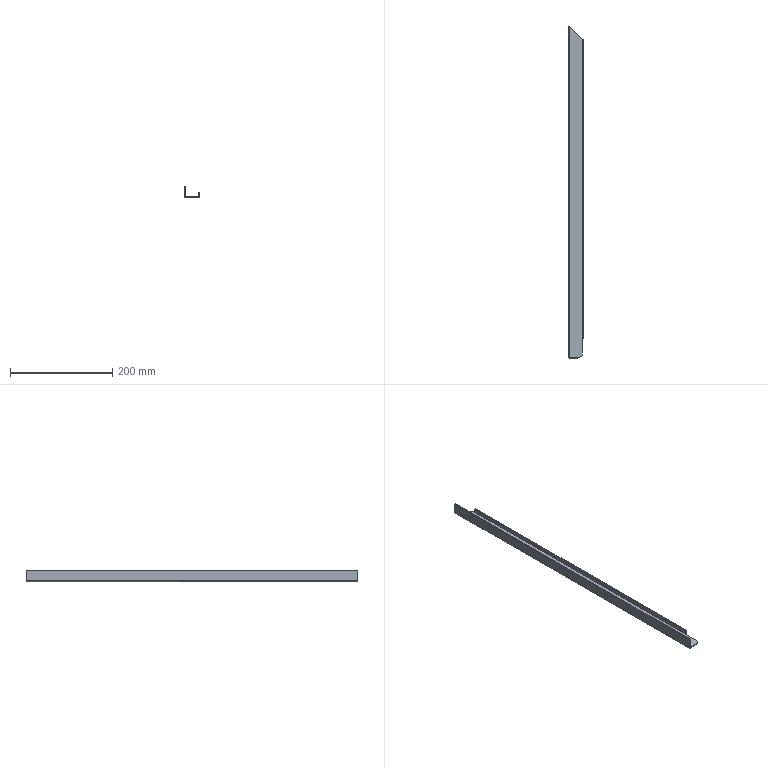Part | STEP file | Rear Closing Plate Door Frame Right | 1 solid | 21 faces | box 30 x 650.24 x 22 mm | volume 72183 mm3 | plane 14 | cylinder 5 | spline 2 | commonest cylinder face diameters 0.2 x2 4.2 x2 20 x1
STEP:
#1=CARTESIAN_POINT('',(24.549,-282.608,2.));
#2=VERTEX_POINT('',#1);
#3=CARTESIAN_POINT('',(14.549,-292.608,2.));
#4=VERTEX_POINT('',#3);
#5=CARTESIAN_POINT('',(14.549,-282.608,2.));
#6=DIRECTION('',(0.,0.,-1.));
#7=DIRECTION('',(-1.,0.,0.));
#8=AXIS2_PLACEMENT_3D('',#5,#6,#7);
#9=CIRCLE('',#8,10.);
#10=EDGE_CURVE('',#2,#4,#9,.T.);
#11=ORIENTED_EDGE('',*,*,#10,.F.);
#12=CARTESIAN_POINT('',(24.549,-254.608,2.));
#13=VERTEX_POINT('',#12);
#14=CARTESIAN_POINT('',(24.549,0.,2.));
#15=DIRECTION('',(0.,-1.,0.));
#16=VECTOR('',#15,1000.);
#17=LINE('',#14,#16);
#18=EDGE_CURVE('',#13,#2,#17,.T.);
#19=ORIENTED_EDGE('',*,*,#18,.F.);
#20=CARTESIAN_POINT('',(24.649,-254.608,2.));
#21=VERTEX_POINT('',#20);
#22=CARTESIAN_POINT('',(667.249,-254.608,2.));
#23=DIRECTION('',(1.,0.,0.));
#24=VECTOR('',#23,1000.);
#25=LINE('',#22,#24);
#26=EDGE_CURVE('',#13,#21,#25,.T.);
#27=ORIENTED_EDGE('',*,*,#26,.T.);
#28=CARTESIAN_POINT('',(24.649,331.492,2.));
#29=VERTEX_POINT('',#28);
#30=CARTESIAN_POINT('',(24.649,0.,2.));
#31=DIRECTION('',(0.,-1.,0.));
#32=VECTOR('',#31,1000.);
#33=LINE('',#30,#32);
#34=EDGE_CURVE('',#29,#21,#33,.T.);
#35=ORIENTED_EDGE('',*,*,#34,.F.);
#36=CARTESIAN_POINT('',(-1.151,357.292,2.));
#37=VERTEX_POINT('',#36);
#38=CARTESIAN_POINT('',(-1.151,357.292,2.));
#39=DIRECTION('',(0.7071,-0.7071,0.));
#40=VECTOR('',#39,1000.);
#41=LINE('',#38,#40);
#42=EDGE_CURVE('',#37,#29,#41,.T.);
#43=ORIENTED_EDGE('',*,*,#42,.F.);
#44=CARTESIAN_POINT('',(-1.151,-292.608,2.));
#45=VERTEX_POINT('',#44);
#46=CARTESIAN_POINT('',(-1.151,0.,2.));
#47=DIRECTION('',(0.,1.,0.));
#48=VECTOR('',#47,1000.);
#49=LINE('',#46,#48);
#50=EDGE_CURVE('',#45,#37,#49,.T.);
#51=ORIENTED_EDGE('',*,*,#50,.F.);
#52=CARTESIAN_POINT('',(0.,-292.608,2.));
#53=DIRECTION('',(-1.,0.,0.));
#54=VECTOR('',#53,1000.);
#55=LINE('',#52,#54);
#56=EDGE_CURVE('',#4,#45,#55,.T.);
#57=ORIENTED_EDGE('',*,*,#56,.F.);
#58=EDGE_LOOP('',(#11,#19,#27,#35,#43,#51,#57));
#59=FACE_OUTER_BOUND('',#58,.T.);
#60=CARTESIAN_POINT('',(0.,0.,2.));
#61=DIRECTION('',(0.,0.,-1.));
#62=DIRECTION('',(-1.,0.,0.));
#63=AXIS2_PLACEMENT_3D('',#60,#61,#62);
#64=PLANE('',#63);
#65=ADVANCED_FACE('',(#59),#64,.F.);
#66=CARTESIAN_POINT('',(14.549,-292.608,0.));
#67=VERTEX_POINT('',#66);
#68=CARTESIAN_POINT('',(14.549,-292.608,0.));
#69=DIRECTION('',(0.,0.,-1.));
#70=VECTOR('',#69,1000.);
#71=LINE('',#68,#70);
#72=EDGE_CURVE('',#4,#67,#71,.T.);
#73=ORIENTED_EDGE('',*,*,#72,.F.);
#74=ORIENTED_EDGE('',*,*,#56,.T.);
#75=CARTESIAN_POINT('',(-1.251,-292.608,2.1));
#76=VERTEX_POINT('',#75);
#77=CARTESIAN_POINT('',(-1.151,-292.608,2.1));
#78=DIRECTION('',(0.,1.,0.));
#79=DIRECTION('',(-1.,0.,0.));
#80=AXIS2_PLACEMENT_3D('',#77,#78,#79);
#81=CIRCLE('',#80,0.1);
#82=EDGE_CURVE('',#45,#76,#81,.T.);
#83=ORIENTED_EDGE('',*,*,#82,.T.);
#84=CARTESIAN_POINT('',(-1.251,-292.608,22.));
#85=VERTEX_POINT('',#84);
#86=CARTESIAN_POINT('',(-1.251,-292.608,22.));
#87=DIRECTION('',(0.,0.,-1.));
#88=VECTOR('',#87,1000.);
#89=LINE('',#86,#88);
#90=EDGE_CURVE('',#85,#76,#89,.T.);
#91=ORIENTED_EDGE('',*,*,#90,.F.);
#92=CARTESIAN_POINT('',(-3.251,-292.608,22.));
#93=VERTEX_POINT('',#92);
#94=CARTESIAN_POINT('',(-3.251,-292.608,22.));
#95=DIRECTION('',(-1.,0.,0.));
#96=VECTOR('',#95,1000.);
#97=LINE('',#94,#96);
#98=EDGE_CURVE('',#85,#93,#97,.T.);
#99=ORIENTED_EDGE('',*,*,#98,.T.);
#100=CARTESIAN_POINT('',(-3.251,-292.608,2.1));
#101=VERTEX_POINT('',#100);
#102=CARTESIAN_POINT('',(-3.251,-292.608,22.));
#103=DIRECTION('',(0.,0.,-1.));
#104=VECTOR('',#103,1000.);
#105=LINE('',#102,#104);
#106=EDGE_CURVE('',#93,#101,#105,.T.);
#107=ORIENTED_EDGE('',*,*,#106,.T.);
#108=CARTESIAN_POINT('',(-1.151,-292.608,0.));
#109=VERTEX_POINT('',#108);
#110=CARTESIAN_POINT('',(-1.151,-292.608,2.1));
#111=DIRECTION('',(0.,1.,0.));
#112=DIRECTION('',(-1.,0.,0.));
#113=AXIS2_PLACEMENT_3D('',#110,#111,#112);
#114=CIRCLE('',#113,2.1);
#115=EDGE_CURVE('',#109,#101,#114,.T.);
#116=ORIENTED_EDGE('',*,*,#115,.F.);
#117=CARTESIAN_POINT('',(24.549,-292.608,0.));
#118=DIRECTION('',(-1.,0.,0.));
#119=VECTOR('',#118,1000.);
#120=LINE('',#117,#119);
#121=EDGE_CURVE('',#67,#109,#120,.T.);
#122=ORIENTED_EDGE('',*,*,#121,.F.);
#123=EDGE_LOOP('',(#73,#74,#83,#91,#99,#107,#116,#122));
#124=FACE_OUTER_BOUND('',#123,.T.);
#125=CARTESIAN_POINT('',(24.549,-292.608,0.));
#126=DIRECTION('',(0.,1.,0.));
#127=DIRECTION('',(-1.,0.,0.));
#128=AXIS2_PLACEMENT_3D('',#125,#126,#127);
#129=PLANE('',#128);
#130=ADVANCED_FACE('',(#124),#129,.F.);
#131=CARTESIAN_POINT('',(24.549,-282.608,0.));
#132=VERTEX_POINT('',#131);
#133=CARTESIAN_POINT('',(14.549,-282.608,0.));
#134=DIRECTION('',(0.,0.,1.));
#135=DIRECTION('',(-1.,0.,0.));
#136=AXIS2_PLACEMENT_3D('',#133,#134,#135);
#137=CIRCLE('',#136,10.);
#138=EDGE_CURVE('',#67,#132,#137,.T.);
#139=ORIENTED_EDGE('',*,*,#138,.T.);
#140=CARTESIAN_POINT('',(24.549,-282.608,0.));
#141=DIRECTION('',(0.,0.,1.));
#142=VECTOR('',#141,1000.);
#143=LINE('',#140,#142);
#144=EDGE_CURVE('',#132,#2,#143,.T.);
#145=ORIENTED_EDGE('',*,*,#144,.T.);
#146=ORIENTED_EDGE('',*,*,#10,.T.);
#147=ORIENTED_EDGE('',*,*,#72,.T.);
#148=EDGE_LOOP('',(#139,#145,#146,#147));
#149=FACE_OUTER_BOUND('',#148,.T.);
#150=CARTESIAN_POINT('',(14.549,-282.608,0.));
#151=DIRECTION('',(0.,0.,-1.));
#152=DIRECTION('',(-1.,0.,0.));
#153=AXIS2_PLACEMENT_3D('',#150,#151,#152);
#154=CYLINDRICAL_SURFACE('',#153,10.);
#155=ADVANCED_FACE('',(#149),#154,.T.);
#156=ORIENTED_EDGE('',*,*,#144,.F.);
#157=CARTESIAN_POINT('',(24.549,-254.608,0.));
#158=VERTEX_POINT('',#157);
#159=CARTESIAN_POINT('',(24.549,-254.608,0.));
#160=DIRECTION('',(0.,-1.,0.));
#161=VECTOR('',#160,1000.);
#162=LINE('',#159,#161);
#163=EDGE_CURVE('',#158,#132,#162,.T.);
#164=ORIENTED_EDGE('',*,*,#163,.F.);
#165=CARTESIAN_POINT('',(24.549,-254.608,0.));
#166=DIRECTION('',(0.,0.,-1.));
#167=VECTOR('',#166,1000.);
#168=LINE('',#165,#167);
#169=EDGE_CURVE('',#13,#158,#168,.T.);
#170=ORIENTED_EDGE('',*,*,#169,.F.);
#171=ORIENTED_EDGE('',*,*,#18,.T.);
#172=EDGE_LOOP('',(#156,#164,#170,#171));
#173=FACE_OUTER_BOUND('',#172,.T.);
#174=CARTESIAN_POINT('',(24.549,-254.608,0.));
#175=DIRECTION('',(-1.,0.,0.));
#176=DIRECTION('',(0.,-1.,0.));
#177=AXIS2_PLACEMENT_3D('',#174,#175,#176);
#178=PLANE('',#177);
#179=ADVANCED_FACE('',(#173),#178,.F.);
#180=ORIENTED_EDGE('',*,*,#34,.T.);
#181=CARTESIAN_POINT('',(24.749,-254.608,2.1));
#182=VERTEX_POINT('',#181);
#183=CARTESIAN_POINT('',(24.649,-254.608,2.1));
#184=DIRECTION('',(0.,1.,0.));
#185=DIRECTION('',(1.,0.,0.));
#186=AXIS2_PLACEMENT_3D('',#183,#184,#185);
#187=CIRCLE('',#186,0.1);
#188=EDGE_CURVE('',#182,#21,#187,.T.);
#189=ORIENTED_EDGE('',*,*,#188,.F.);
#190=CARTESIAN_POINT('',(24.749,329.392,2.1));
#191=VERTEX_POINT('',#190);
#192=CARTESIAN_POINT('',(24.749,0.,2.1));
#193=DIRECTION('',(0.,-1.,0.));
#194=VECTOR('',#193,1000.);
#195=LINE('',#192,#194);
#196=EDGE_CURVE('',#191,#182,#195,.T.);
#197=ORIENTED_EDGE('',*,*,#196,.F.);
#198=CARTESIAN_POINT('',(24.649,331.492,2.));
#199=CARTESIAN_POINT('',(24.716,330.092,2.));
#200=CARTESIAN_POINT('',(24.749,329.392,2.05));
#201=CARTESIAN_POINT('',(24.749,329.392,2.1));
#202=(BOUNDED_CURVE()B_SPLINE_CURVE(3,(#198,#199,#200,#201),.UNSPECIFIED.,.F.,.F.)B_SPLINE_CURVE_WITH_KNOTS((4,4),(0.,0.002112),.UNSPECIFIED.)CURVE()GEOMETRIC_REPRESENTATION_ITEM()RATIONAL_B_SPLINE_CURVE((0.5,0.5,0.6667,1.))REPRESENTATION_ITEM(''));
#203=EDGE_CURVE('',#29,#191,#202,.T.);
#204=ORIENTED_EDGE('',*,*,#203,.F.);
#205=EDGE_LOOP('',(#180,#189,#197,#204));
#206=FACE_OUTER_BOUND('',#205,.T.);
#207=CARTESIAN_POINT('',(24.649,0.,2.1));
#208=DIRECTION('',(0.,-1.,0.));
#209=DIRECTION('',(1.,0.,0.));
#210=AXIS2_PLACEMENT_3D('',#207,#208,#209);
#211=CYLINDRICAL_SURFACE('',#210,0.1);
#212=ADVANCED_FACE('',(#206),#211,.F.);
#213=ORIENTED_EDGE('',*,*,#42,.T.);
#214=CARTESIAN_POINT('',(24.649,331.492,0.));
#215=VERTEX_POINT('',#214);
#216=CARTESIAN_POINT('',(24.649,331.492,0.));
#217=DIRECTION('',(0.,0.,1.));
#218=VECTOR('',#217,1000.);
#219=LINE('',#216,#218);
#220=EDGE_CURVE('',#215,#29,#219,.T.);
#221=ORIENTED_EDGE('',*,*,#220,.F.);
#222=CARTESIAN_POINT('',(-1.151,357.292,0.));
#223=VERTEX_POINT('',#222);
#224=CARTESIAN_POINT('',(-1.251,357.392,0.));
#225=DIRECTION('',(0.7071,-0.7071,0.));
#226=VECTOR('',#225,1000.);
#227=LINE('',#224,#226);
#228=EDGE_CURVE('',#223,#215,#227,.T.);
#229=ORIENTED_EDGE('',*,*,#228,.F.);
#230=CARTESIAN_POINT('',(-1.151,357.292,0.));
#231=DIRECTION('',(0.,0.,-1.));
#232=VECTOR('',#231,1000.);
#233=LINE('',#230,#232);
#234=EDGE_CURVE('',#37,#223,#233,.T.);
#235=ORIENTED_EDGE('',*,*,#234,.F.);
#236=EDGE_LOOP('',(#213,#221,#229,#235));
#237=FACE_OUTER_BOUND('',#236,.T.);
#238=CARTESIAN_POINT('',(-1.251,357.392,0.));
#239=DIRECTION('',(-0.7071,-0.7071,0.));
#240=DIRECTION('',(0.7071,-0.7071,0.));
#241=AXIS2_PLACEMENT_3D('',#238,#239,#240);
#242=PLANE('',#241);
#243=ADVANCED_FACE('',(#237),#242,.F.);
#244=CARTESIAN_POINT('',(-1.251,357.392,2.1));
#245=VERTEX_POINT('',#244);
#246=CARTESIAN_POINT('',(-1.251,359.392,2.1));
#247=DIRECTION('',(0.,1.,0.));
#248=VECTOR('',#247,1000.);
#249=LINE('',#246,#248);
#250=EDGE_CURVE('',#76,#245,#249,.T.);
#251=ORIENTED_EDGE('',*,*,#250,.F.);
#252=ORIENTED_EDGE('',*,*,#82,.F.);
#253=ORIENTED_EDGE('',*,*,#50,.T.);
#254=CARTESIAN_POINT('',(-1.251,357.392,2.1));
#255=CARTESIAN_POINT('',(-1.251,357.392,2.093));
#256=CARTESIAN_POINT('',(-1.251,357.399,2.09));
#257=CARTESIAN_POINT('',(-1.25,357.41,2.084));
#258=CARTESIAN_POINT('',(-1.249,357.416,2.081));
#259=CARTESIAN_POINT('',(-1.248,357.434,2.074));
#260=CARTESIAN_POINT('',(-1.247,357.446,2.07));
#261=CARTESIAN_POINT('',(-1.243,357.483,2.059));
#262=CARTESIAN_POINT('',(-1.239,357.508,2.052));
#263=CARTESIAN_POINT('',(-1.231,357.557,2.039));
#264=CARTESIAN_POINT('',(-1.226,357.581,2.033));
#265=CARTESIAN_POINT('',(-1.216,357.611,2.024));
#266=CARTESIAN_POINT('',(-1.214,357.616,2.022));
#267=CARTESIAN_POINT('',(-1.208,357.627,2.017));
#268=CARTESIAN_POINT('',(-1.203,357.633,2.014));
#269=CARTESIAN_POINT('',(-1.192,357.628,2.009));
#270=CARTESIAN_POINT('',(-1.189,357.622,2.008));
#271=CARTESIAN_POINT('',(-1.185,357.61,2.006));
#272=CARTESIAN_POINT('',(-1.183,357.604,2.005));
#273=CARTESIAN_POINT('',(-1.168,357.548,2.001));
#274=CARTESIAN_POINT('',(-1.165,357.496,2.001));
#275=CARTESIAN_POINT('',(-1.157,357.394,2.));
#276=CARTESIAN_POINT('',(-1.154,357.343,2.));
#277=CARTESIAN_POINT('',(-1.151,357.292,2.));
#278=B_SPLINE_CURVE_WITH_KNOTS('',3,(#254,#255,#256,#257,#258,#259,#260,#261,#262,#263,#264,#265,#266,#267,#268,#269,#270,#271,#272,#273,#274,#275,#276,#277),.UNSPECIFIED.,.F.,.F.,(4,2,2,2,2,2,2,2,2,2,2,4),(0.,0.00001954,0.00003907,0.00007815,0.0001563,0.0002344,0.000254,0.0002735,0.0002931,0.0003126,0.0004689,0.0006252),.UNSPECIFIED.);
#279=EDGE_CURVE('',#245,#37,#278,.T.);
#280=ORIENTED_EDGE('',*,*,#279,.F.);
#281=EDGE_LOOP('',(#251,#252,#253,#280));
#282=FACE_OUTER_BOUND('',#281,.T.);
#283=CARTESIAN_POINT('',(-1.151,359.392,2.1));
#284=DIRECTION('',(0.,1.,0.));
#285=DIRECTION('',(-1.,0.,0.));
#286=AXIS2_PLACEMENT_3D('',#283,#284,#285);
#287=CYLINDRICAL_SURFACE('',#286,0.1);
#288=ADVANCED_FACE('',(#282),#287,.F.);
#289=CARTESIAN_POINT('',(24.649,-254.608,0.));
#290=VERTEX_POINT('',#289);
#291=CARTESIAN_POINT('',(24.649,0.,0.));
#292=DIRECTION('',(0.,-1.,0.));
#293=VECTOR('',#292,1000.);
#294=LINE('',#291,#293);
#295=EDGE_CURVE('',#215,#290,#294,.T.);
#296=ORIENTED_EDGE('',*,*,#295,.T.);
#297=CARTESIAN_POINT('',(0.,-254.608,0.));
#298=DIRECTION('',(-1.,0.,0.));
#299=VECTOR('',#298,1000.);
#300=LINE('',#297,#299);
#301=EDGE_CURVE('',#290,#158,#300,.T.);
#302=ORIENTED_EDGE('',*,*,#301,.T.);
#303=ORIENTED_EDGE('',*,*,#163,.T.);
#304=ORIENTED_EDGE('',*,*,#138,.F.);
#305=ORIENTED_EDGE('',*,*,#121,.T.);
#306=CARTESIAN_POINT('',(-1.151,0.,0.));
#307=DIRECTION('',(0.,1.,0.));
#308=VECTOR('',#307,1000.);
#309=LINE('',#306,#308);
#310=EDGE_CURVE('',#109,#223,#309,.T.);
#311=ORIENTED_EDGE('',*,*,#310,.T.);
#312=ORIENTED_EDGE('',*,*,#228,.T.);
#313=EDGE_LOOP('',(#296,#302,#303,#304,#305,#311,#312));
#314=FACE_OUTER_BOUND('',#313,.T.);
#315=CARTESIAN_POINT('',(0.,0.,0.));
#316=DIRECTION('',(0.,0.,-1.));
#317=DIRECTION('',(-1.,0.,0.));
#318=AXIS2_PLACEMENT_3D('',#315,#316,#317);
#319=PLANE('',#318);
#320=ADVANCED_FACE('',(#314),#319,.T.);
#321=ORIENTED_EDGE('',*,*,#26,.F.);
#322=ORIENTED_EDGE('',*,*,#169,.T.);
#323=ORIENTED_EDGE('',*,*,#301,.F.);
#324=CARTESIAN_POINT('',(26.749,-254.608,2.1));
#325=VERTEX_POINT('',#324);
#326=CARTESIAN_POINT('',(24.649,-254.608,2.1));
#327=DIRECTION('',(0.,1.,0.));
#328=DIRECTION('',(1.,0.,0.));
#329=AXIS2_PLACEMENT_3D('',#326,#327,#328);
#330=CIRCLE('',#329,2.1);
#331=EDGE_CURVE('',#325,#290,#330,.T.);
#332=ORIENTED_EDGE('',*,*,#331,.F.);
#333=CARTESIAN_POINT('',(26.749,-254.608,10.));
#334=VERTEX_POINT('',#333);
#335=CARTESIAN_POINT('',(26.749,-254.608,22.));
#336=DIRECTION('',(0.,0.,1.));
#337=VECTOR('',#336,1000.);
#338=LINE('',#335,#337);
#339=EDGE_CURVE('',#325,#334,#338,.T.);
#340=ORIENTED_EDGE('',*,*,#339,.T.);
#341=CARTESIAN_POINT('',(24.749,-254.608,10.));
#342=VERTEX_POINT('',#341);
#343=CARTESIAN_POINT('',(26.749,-254.608,10.));
#344=DIRECTION('',(-1.,0.,0.));
#345=VECTOR('',#344,1000.);
#346=LINE('',#343,#345);
#347=EDGE_CURVE('',#334,#342,#346,.T.);
#348=ORIENTED_EDGE('',*,*,#347,.T.);
#349=CARTESIAN_POINT('',(24.749,-254.608,22.));
#350=DIRECTION('',(0.,0.,-1.));
#351=VECTOR('',#350,1000.);
#352=LINE('',#349,#351);
#353=EDGE_CURVE('',#342,#182,#352,.T.);
#354=ORIENTED_EDGE('',*,*,#353,.T.);
#355=ORIENTED_EDGE('',*,*,#188,.T.);
#356=EDGE_LOOP('',(#321,#322,#323,#332,#340,#348,#354,#355));
#357=FACE_OUTER_BOUND('',#356,.T.);
#358=CARTESIAN_POINT('',(667.249,-254.608,0.));
#359=DIRECTION('',(0.,1.,0.));
#360=DIRECTION('',(0.,0.,1.));
#361=AXIS2_PLACEMENT_3D('',#358,#359,#360);
#362=PLANE('',#361);
#363=ADVANCED_FACE('',(#357),#362,.F.);
#364=ORIENTED_EDGE('',*,*,#203,.T.);
#365=CARTESIAN_POINT('',(26.749,329.392,2.1));
#366=VERTEX_POINT('',#365);
#367=CARTESIAN_POINT('',(25.749,329.392,2.1));
#368=DIRECTION('',(-1.,0.,0.));
#369=VECTOR('',#368,1000.);
#370=LINE('',#367,#369);
#371=EDGE_CURVE('',#366,#191,#370,.T.);
#372=ORIENTED_EDGE('',*,*,#371,.F.);
#373=CARTESIAN_POINT('',(24.649,331.492,0.));
#374=CARTESIAN_POINT('',(26.049,330.092,0.));
#375=CARTESIAN_POINT('',(26.749,329.392,1.05));
#376=CARTESIAN_POINT('',(26.749,329.392,2.1));
#377=(BOUNDED_CURVE()B_SPLINE_CURVE(3,(#373,#374,#375,#376),.UNSPECIFIED.,.F.,.F.)B_SPLINE_CURVE_WITH_KNOTS((4,4),(0.,0.003971),.UNSPECIFIED.)CURVE()GEOMETRIC_REPRESENTATION_ITEM()RATIONAL_B_SPLINE_CURVE((0.5,0.5,0.6667,1.))REPRESENTATION_ITEM(''));
#378=EDGE_CURVE('',#215,#366,#377,.T.);
#379=ORIENTED_EDGE('',*,*,#378,.F.);
#380=ORIENTED_EDGE('',*,*,#220,.T.);
#381=EDGE_LOOP('',(#364,#372,#379,#380));
#382=FACE_OUTER_BOUND('',#381,.T.);
#383=CARTESIAN_POINT('',(26.749,329.392,2.1));
#384=CARTESIAN_POINT('',(26.082,329.392,2.1));
#385=CARTESIAN_POINT('',(25.416,329.392,2.1));
#386=CARTESIAN_POINT('',(24.749,329.392,2.1));
#387=CARTESIAN_POINT('',(26.749,329.392,6.3));
#388=CARTESIAN_POINT('',(26.082,329.392,4.967));
#389=CARTESIAN_POINT('',(25.416,329.392,3.633));
#390=CARTESIAN_POINT('',(24.749,329.392,2.3));
#391=CARTESIAN_POINT('',(22.549,333.592,6.3));
#392=CARTESIAN_POINT('',(23.216,333.592,4.967));
#393=CARTESIAN_POINT('',(23.882,333.592,3.633));
#394=CARTESIAN_POINT('',(24.549,333.592,2.3));
#395=CARTESIAN_POINT('',(22.549,333.592,2.1));
#396=CARTESIAN_POINT('',(23.216,333.592,2.1));
#397=CARTESIAN_POINT('',(23.882,333.592,2.1));
#398=CARTESIAN_POINT('',(24.549,333.592,2.1));
#399=CARTESIAN_POINT('',(22.549,333.592,-2.1));
#400=CARTESIAN_POINT('',(23.216,333.592,-0.7667));
#401=CARTESIAN_POINT('',(23.882,333.592,0.5667));
#402=CARTESIAN_POINT('',(24.549,333.592,1.9));
#403=CARTESIAN_POINT('',(26.749,329.392,-2.1));
#404=CARTESIAN_POINT('',(26.082,329.392,-0.7667));
#405=CARTESIAN_POINT('',(25.416,329.392,0.5667));
#406=CARTESIAN_POINT('',(24.749,329.392,1.9));
#407=CARTESIAN_POINT('',(26.749,329.392,2.1));
#408=CARTESIAN_POINT('',(26.082,329.392,2.1));
#409=CARTESIAN_POINT('',(25.416,329.392,2.1));
#410=CARTESIAN_POINT('',(24.749,329.392,2.1));
#411=(BOUNDED_SURFACE()B_SPLINE_SURFACE(3,3,((#383,#384,#385,#386),(#387,#388,#389,#390),(#391,#392,#393,#394),(#395,#396,#397,#398),(#399,#400,#401,#402),(#403,#404,#405,#406),(#407,#408,#409,#410)),.UNSPECIFIED.,.T.,.F.,.F.)B_SPLINE_SURFACE_WITH_KNOTS((4,3,4),(4,4),(0.,0.5,1.),(0.,1.),.UNSPECIFIED.)GEOMETRIC_REPRESENTATION_ITEM()RATIONAL_B_SPLINE_SURFACE(((1.,1.,1.,1.),(0.3333,0.3333,0.3333,0.3333),(0.3333,0.3333,0.3333,0.3333),(1.,1.,1.,1.),(0.3333,0.3333,0.3333,0.3333),(0.3333,0.3333,0.3333,0.3333),(1.,1.,1.,1.)))REPRESENTATION_ITEM('')SURFACE());
#412=ADVANCED_FACE('',(#382),#411,.F.);
#413=CARTESIAN_POINT('',(24.749,329.392,10.));
#414=VERTEX_POINT('',#413);
#415=CARTESIAN_POINT('',(24.749,329.392,10.));
#416=DIRECTION('',(0.,-1.,0.));
#417=VECTOR('',#416,1000.);
#418=LINE('',#415,#417);
#419=EDGE_CURVE('',#414,#342,#418,.T.);
#420=ORIENTED_EDGE('',*,*,#419,.F.);
#421=CARTESIAN_POINT('',(24.749,329.392,22.));
#422=DIRECTION('',(0.,0.,1.));
#423=VECTOR('',#422,1000.);
#424=LINE('',#421,#423);
#425=EDGE_CURVE('',#191,#414,#424,.T.);
#426=ORIENTED_EDGE('',*,*,#425,.F.);
#427=ORIENTED_EDGE('',*,*,#196,.T.);
#428=ORIENTED_EDGE('',*,*,#353,.F.);
#429=EDGE_LOOP('',(#420,#426,#427,#428));
#430=FACE_OUTER_BOUND('',#429,.T.);
#431=CARTESIAN_POINT('',(24.749,329.392,22.));
#432=DIRECTION('',(1.,0.,0.));
#433=DIRECTION('',(0.,1.,0.));
#434=AXIS2_PLACEMENT_3D('',#431,#432,#433);
#435=PLANE('',#434);
#436=ADVANCED_FACE('',(#430),#435,.F.);
#437=ORIENTED_EDGE('',*,*,#279,.T.);
#438=ORIENTED_EDGE('',*,*,#234,.T.);
#439=CARTESIAN_POINT('',(-3.251,357.392,2.1));
#440=VERTEX_POINT('',#439);
#441=CARTESIAN_POINT('',(-3.251,357.392,2.1));
#442=CARTESIAN_POINT('',(-3.251,357.392,1.958));
#443=CARTESIAN_POINT('',(-3.237,357.403,1.816));
#444=CARTESIAN_POINT('',(-3.18,357.435,1.539));
#445=CARTESIAN_POINT('',(-3.138,357.455,1.406));
#446=CARTESIAN_POINT('',(-3.029,357.497,1.15));
#447=CARTESIAN_POINT('',(-2.961,357.519,1.026));
#448=CARTESIAN_POINT('',(-2.803,357.561,0.796));
#449=CARTESIAN_POINT('',(-2.713,357.58,0.6898));
#450=CARTESIAN_POINT('',(-2.513,357.612,0.495));
#451=CARTESIAN_POINT('',(-2.4,357.624,0.4061));
#452=CARTESIAN_POINT('',(-2.163,357.634,0.2546));
#453=CARTESIAN_POINT('',(-2.036,357.632,0.1903));
#454=CARTESIAN_POINT('',(-1.773,357.6,0.08907));
#455=CARTESIAN_POINT('',(-1.637,357.572,0.05272));
#456=CARTESIAN_POINT('',(-1.376,357.468,0.00789));
#457=CARTESIAN_POINT('',(-1.253,357.393,0.));
#458=CARTESIAN_POINT('',(-1.151,357.292,0.));
#459=B_SPLINE_CURVE_WITH_KNOTS('',3,(#441,#442,#443,#444,#445,#446,#447,#448,#449,#450,#451,#452,#453,#454,#455,#456,#457,#458),.UNSPECIFIED.,.F.,.F.,(4,2,2,2,2,2,2,2,4),(0.,0.0004273,0.0008547,0.001282,0.001709,0.002137,0.002564,0.002991,0.003419),.UNSPECIFIED.);
#460=EDGE_CURVE('',#440,#223,#459,.T.);
#461=ORIENTED_EDGE('',*,*,#460,.F.);
#462=CARTESIAN_POINT('',(-2.251,357.392,2.1));
#463=DIRECTION('',(-1.,0.,0.));
#464=VECTOR('',#463,1000.);
#465=LINE('',#462,#464);
#466=EDGE_CURVE('',#245,#440,#465,.T.);
#467=ORIENTED_EDGE('',*,*,#466,.F.);
#468=EDGE_LOOP('',(#437,#438,#461,#467));
#469=FACE_OUTER_BOUND('',#468,.T.);
#470=CARTESIAN_POINT('',(-1.151,357.292,-0.0202));
#471=CARTESIAN_POINT('',(-1.328,357.466,-0.0202));
#472=CARTESIAN_POINT('',(-1.564,357.561,0.003288));
#473=CARTESIAN_POINT('',(-2.071,357.645,0.1713));
#474=CARTESIAN_POINT('',(-2.341,357.636,0.3179));
#475=CARTESIAN_POINT('',(-2.801,357.573,0.7325));
#476=CARTESIAN_POINT('',(-2.988,357.52,0.999));
#477=CARTESIAN_POINT('',(-3.224,357.429,1.559));
#478=CARTESIAN_POINT('',(-3.271,357.392,1.851));
#479=CARTESIAN_POINT('',(-3.271,357.392,2.1));
#480=CARTESIAN_POINT('',(-1.151,357.292,0.));
#481=CARTESIAN_POINT('',(-1.326,357.466,0.));
#482=CARTESIAN_POINT('',(-1.56,357.561,0.02326));
#483=CARTESIAN_POINT('',(-2.063,357.645,0.1897));
#484=CARTESIAN_POINT('',(-2.329,357.636,0.3349));
#485=CARTESIAN_POINT('',(-2.785,357.573,0.7455));
#486=CARTESIAN_POINT('',(-2.971,357.52,1.01));
#487=CARTESIAN_POINT('',(-3.204,357.429,1.565));
#488=CARTESIAN_POINT('',(-3.251,357.392,1.853));
#489=CARTESIAN_POINT('',(-3.251,357.392,2.1));
#490=CARTESIAN_POINT('',(-1.151,357.292,2.));
#491=CARTESIAN_POINT('',(-1.16,357.467,2.));
#492=CARTESIAN_POINT('',(-1.171,357.561,2.001));
#493=CARTESIAN_POINT('',(-1.195,357.645,2.009));
#494=CARTESIAN_POINT('',(-1.207,357.636,2.016));
#495=CARTESIAN_POINT('',(-1.229,357.573,2.035));
#496=CARTESIAN_POINT('',(-1.238,357.52,2.048));
#497=CARTESIAN_POINT('',(-1.249,357.429,2.075));
#498=CARTESIAN_POINT('',(-1.251,357.392,2.088));
#499=CARTESIAN_POINT('',(-1.251,357.392,2.1));
#500=CARTESIAN_POINT('',(-1.151,357.292,2.02));
#501=CARTESIAN_POINT('',(-1.158,357.467,2.02));
#502=CARTESIAN_POINT('',(-1.167,357.561,2.021));
#503=CARTESIAN_POINT('',(-1.186,357.645,2.027));
#504=CARTESIAN_POINT('',(-1.196,357.636,2.033));
#505=CARTESIAN_POINT('',(-1.213,357.573,2.048));
#506=CARTESIAN_POINT('',(-1.22,357.52,2.058));
#507=CARTESIAN_POINT('',(-1.229,357.429,2.08));
#508=CARTESIAN_POINT('',(-1.231,357.392,2.091));
#509=CARTESIAN_POINT('',(-1.231,357.392,2.1));
#510=B_SPLINE_SURFACE_WITH_KNOTS('',1,3,((#470,#471,#472,#473,#474,#475,#476,#477,#478,#479),(#480,#481,#482,#483,#484,#485,#486,#487,#488,#489),(#490,#491,#492,#493,#494,#495,#496,#497,#498,#499),(#500,#501,#502,#503,#504,#505,#506,#507,#508,#509)),.UNSPECIFIED.,.F.,.F.,.F.,(2,1,1,2),(4,2,2,2,4),(-0.0101,0.,1.,1.01),(0.,0.25,0.5,0.75,1.),.UNSPECIFIED.);
#511=ADVANCED_FACE('',(#469),#510,.F.);
#512=ORIENTED_EDGE('',*,*,#90,.T.);
#513=ORIENTED_EDGE('',*,*,#250,.T.);
#514=CARTESIAN_POINT('',(-1.251,357.392,22.));
#515=VERTEX_POINT('',#514);
#516=CARTESIAN_POINT('',(-1.251,357.392,22.));
#517=DIRECTION('',(0.,0.,1.));
#518=VECTOR('',#517,1000.);
#519=LINE('',#516,#518);
#520=EDGE_CURVE('',#245,#515,#519,.T.);
#521=ORIENTED_EDGE('',*,*,#520,.T.);
#522=CARTESIAN_POINT('',(-1.251,359.392,22.));
#523=DIRECTION('',(0.,-1.,0.));
#524=VECTOR('',#523,1000.);
#525=LINE('',#522,#524);
#526=EDGE_CURVE('',#515,#85,#525,.T.);
#527=ORIENTED_EDGE('',*,*,#526,.T.);
#528=EDGE_LOOP('',(#512,#513,#521,#527));
#529=FACE_OUTER_BOUND('',#528,.T.);
#530=CARTESIAN_POINT('',(-1.251,359.392,22.));
#531=DIRECTION('',(1.,0.,0.));
#532=DIRECTION('',(0.,1.,0.));
#533=AXIS2_PLACEMENT_3D('',#530,#531,#532);
#534=PLANE('',#533);
#535=ADVANCED_FACE('',(#529),#534,.T.);
#536=ORIENTED_EDGE('',*,*,#331,.T.);
#537=ORIENTED_EDGE('',*,*,#295,.F.);
#538=ORIENTED_EDGE('',*,*,#378,.T.);
#539=CARTESIAN_POINT('',(26.749,0.,2.1));
#540=DIRECTION('',(0.,-1.,0.));
#541=VECTOR('',#540,1000.);
#542=LINE('',#539,#541);
#543=EDGE_CURVE('',#366,#325,#542,.T.);
#544=ORIENTED_EDGE('',*,*,#543,.T.);
#545=EDGE_LOOP('',(#536,#537,#538,#544));
#546=FACE_OUTER_BOUND('',#545,.T.);
#547=CARTESIAN_POINT('',(24.649,0.,2.1));
#548=DIRECTION('',(0.,-1.,0.));
#549=DIRECTION('',(1.,0.,0.));
#550=AXIS2_PLACEMENT_3D('',#547,#548,#549);
#551=CYLINDRICAL_SURFACE('',#550,2.1);
#552=ADVANCED_FACE('',(#546),#551,.T.);
#553=ORIENTED_EDGE('',*,*,#115,.T.);
#554=CARTESIAN_POINT('',(-3.251,359.392,2.1));
#555=DIRECTION('',(0.,1.,0.));
#556=VECTOR('',#555,1000.);
#557=LINE('',#554,#556);
#558=EDGE_CURVE('',#101,#440,#557,.T.);
#559=ORIENTED_EDGE('',*,*,#558,.T.);
#560=ORIENTED_EDGE('',*,*,#460,.T.);
#561=ORIENTED_EDGE('',*,*,#310,.F.);
#562=EDGE_LOOP('',(#553,#559,#560,#561));
#563=FACE_OUTER_BOUND('',#562,.T.);
#564=CARTESIAN_POINT('',(-1.151,359.392,2.1));
#565=DIRECTION('',(0.,1.,0.));
#566=DIRECTION('',(-1.,0.,0.));
#567=AXIS2_PLACEMENT_3D('',#564,#565,#566);
#568=CYLINDRICAL_SURFACE('',#567,2.1);
#569=ADVANCED_FACE('',(#563),#568,.T.);
#570=ORIENTED_EDGE('',*,*,#425,.T.);
#571=CARTESIAN_POINT('',(26.749,329.392,10.));
#572=VERTEX_POINT('',#571);
#573=CARTESIAN_POINT('',(26.749,329.392,10.));
#574=DIRECTION('',(-1.,0.,0.));
#575=VECTOR('',#574,1000.);
#576=LINE('',#573,#575);
#577=EDGE_CURVE('',#572,#414,#576,.T.);
#578=ORIENTED_EDGE('',*,*,#577,.F.);
#579=CARTESIAN_POINT('',(26.749,329.392,22.));
#580=DIRECTION('',(0.,0.,1.));
#581=VECTOR('',#580,1000.);
#582=LINE('',#579,#581);
#583=EDGE_CURVE('',#366,#572,#582,.T.);
#584=ORIENTED_EDGE('',*,*,#583,.F.);
#585=ORIENTED_EDGE('',*,*,#371,.T.);
#586=EDGE_LOOP('',(#570,#578,#584,#585));
#587=FACE_OUTER_BOUND('',#586,.T.);
#588=CARTESIAN_POINT('',(26.749,329.392,22.));
#589=DIRECTION('',(0.,-1.,0.));
#590=DIRECTION('',(1.,0.,0.));
#591=AXIS2_PLACEMENT_3D('',#588,#589,#590);
#592=PLANE('',#591);
#593=ADVANCED_FACE('',(#587),#592,.F.);
#594=ORIENTED_EDGE('',*,*,#347,.F.);
#595=CARTESIAN_POINT('',(26.749,329.392,10.));
#596=DIRECTION('',(0.,1.,0.));
#597=VECTOR('',#596,1000.);
#598=LINE('',#595,#597);
#599=EDGE_CURVE('',#334,#572,#598,.T.);
#600=ORIENTED_EDGE('',*,*,#599,.T.);
#601=ORIENTED_EDGE('',*,*,#577,.T.);
#602=ORIENTED_EDGE('',*,*,#419,.T.);
#603=EDGE_LOOP('',(#594,#600,#601,#602));
#604=FACE_OUTER_BOUND('',#603,.T.);
#605=CARTESIAN_POINT('',(26.749,329.392,10.));
#606=DIRECTION('',(0.,0.,1.));
#607=DIRECTION('',(1.,0.,0.));
#608=AXIS2_PLACEMENT_3D('',#605,#606,#607);
#609=PLANE('',#608);
#610=ADVANCED_FACE('',(#604),#609,.T.);
#611=ORIENTED_EDGE('',*,*,#520,.F.);
#612=ORIENTED_EDGE('',*,*,#466,.T.);
#613=CARTESIAN_POINT('',(-3.251,357.392,22.));
#614=VERTEX_POINT('',#613);
#615=CARTESIAN_POINT('',(-3.251,357.392,22.));
#616=DIRECTION('',(0.,0.,-1.));
#617=VECTOR('',#616,1000.);
#618=LINE('',#615,#617);
#619=EDGE_CURVE('',#614,#440,#618,.T.);
#620=ORIENTED_EDGE('',*,*,#619,.F.);
#621=CARTESIAN_POINT('',(-3.251,357.392,22.));
#622=DIRECTION('',(-1.,0.,0.));
#623=VECTOR('',#622,1000.);
#624=LINE('',#621,#623);
#625=EDGE_CURVE('',#515,#614,#624,.T.);
#626=ORIENTED_EDGE('',*,*,#625,.F.);
#627=EDGE_LOOP('',(#611,#612,#620,#626));
#628=FACE_OUTER_BOUND('',#627,.T.);
#629=CARTESIAN_POINT('',(-3.251,357.392,22.));
#630=DIRECTION('',(0.,-1.,0.));
#631=DIRECTION('',(1.,0.,0.));
#632=AXIS2_PLACEMENT_3D('',#629,#630,#631);
#633=PLANE('',#632);
#634=ADVANCED_FACE('',(#628),#633,.F.);
#635=ORIENTED_EDGE('',*,*,#625,.T.);
#636=CARTESIAN_POINT('',(-3.251,359.392,22.));
#637=DIRECTION('',(0.,-1.,0.));
#638=VECTOR('',#637,1000.);
#639=LINE('',#636,#638);
#640=EDGE_CURVE('',#614,#93,#639,.T.);
#641=ORIENTED_EDGE('',*,*,#640,.T.);
#642=ORIENTED_EDGE('',*,*,#98,.F.);
#643=ORIENTED_EDGE('',*,*,#526,.F.);
#644=EDGE_LOOP('',(#635,#641,#642,#643));
#645=FACE_OUTER_BOUND('',#644,.T.);
#646=CARTESIAN_POINT('',(-3.251,359.392,22.));
#647=DIRECTION('',(0.,0.,1.));
#648=DIRECTION('',(1.,0.,0.));
#649=AXIS2_PLACEMENT_3D('',#646,#647,#648);
#650=PLANE('',#649);
#651=ADVANCED_FACE('',(#645),#650,.T.);
#652=ORIENTED_EDGE('',*,*,#583,.T.);
#653=ORIENTED_EDGE('',*,*,#599,.F.);
#654=ORIENTED_EDGE('',*,*,#339,.F.);
#655=ORIENTED_EDGE('',*,*,#543,.F.);
#656=EDGE_LOOP('',(#652,#653,#654,#655));
#657=FACE_OUTER_BOUND('',#656,.T.);
#658=CARTESIAN_POINT('',(26.749,329.392,22.));
#659=DIRECTION('',(1.,0.,0.));
#660=DIRECTION('',(0.,1.,0.));
#661=AXIS2_PLACEMENT_3D('',#658,#659,#660);
#662=PLANE('',#661);
#663=ADVANCED_FACE('',(#657),#662,.T.);
#664=ORIENTED_EDGE('',*,*,#558,.F.);
#665=ORIENTED_EDGE('',*,*,#106,.F.);
#666=ORIENTED_EDGE('',*,*,#640,.F.);
#667=ORIENTED_EDGE('',*,*,#619,.T.);
#668=EDGE_LOOP('',(#664,#665,#666,#667));
#669=FACE_OUTER_BOUND('',#668,.T.);
#670=CARTESIAN_POINT('',(-3.251,359.392,22.));
#671=DIRECTION('',(1.,0.,0.));
#672=DIRECTION('',(0.,1.,0.));
#673=AXIS2_PLACEMENT_3D('',#670,#671,#672);
#674=PLANE('',#673);
#675=ADVANCED_FACE('',(#669),#674,.F.);
#676=CLOSED_SHELL('',(#65,#130,#155,#179,#212,#243,#288,#320,#363,#412,#436,#511,#535,#552,#569,#593,#610,#634,#651,#663,#675));
#677=MANIFOLD_SOLID_BREP('',#676);
#678=CARTESIAN_POINT('',(0.,0.,0.));
#679=DIRECTION('',(0.,0.,1.));
#680=DIRECTION('',(1.,0.,0.));
#681=AXIS2_PLACEMENT_3D('',#678,#679,#680);
#682=(LENGTH_UNIT()NAMED_UNIT(*)SI_UNIT(.MILLI.,.METRE.));
#683=UNCERTAINTY_MEASURE_WITH_UNIT(LENGTH_MEASURE(0.00001),#682,'','');
#684=(NAMED_UNIT(*)PLANE_ANGLE_UNIT()SI_UNIT($,.RADIAN.));
#685=(NAMED_UNIT(*)SI_UNIT($,.STERADIAN.)SOLID_ANGLE_UNIT());
#686=(GEOMETRIC_REPRESENTATION_CONTEXT(3)GLOBAL_UNCERTAINTY_ASSIGNED_CONTEXT((#683))GLOBAL_UNIT_ASSIGNED_CONTEXT((#682,#684,#685))REPRESENTATION_CONTEXT('',''));
#687=ADVANCED_BREP_SHAPE_REPRESENTATION('',(#677,#681),#686);